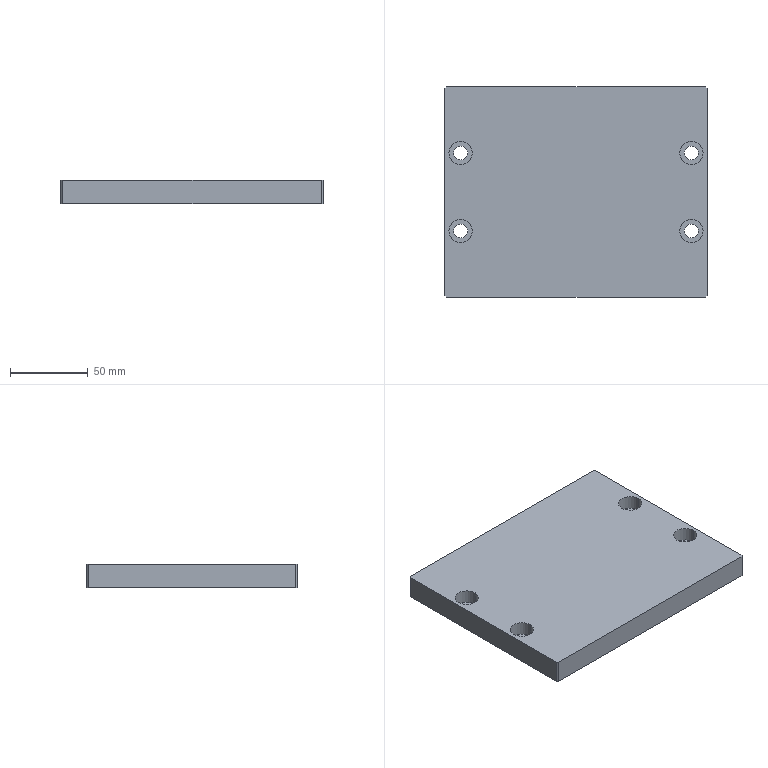Part | SolidWorks | features Chamfer 1, Extrusion 1, HoleWzd 1 | 1 solid | 30 faces | box 168 x 135 x 15 mm | volume 332281 mm3 | cylinder 16 | plane 14 | commonest cylinder face diameters 9 x8 15 x8
STEP:
#1=CARTESIAN_POINT('',(-81.5,25.,6.));
#2=VERTEX_POINT('',#1);
#3=CARTESIAN_POINT('',(-66.5,25.,6.));
#4=VERTEX_POINT('',#3);
#5=CARTESIAN_POINT('',(-74.,25.,6.));
#6=DIRECTION('',(0.,0.,1.));
#7=DIRECTION('',(1.,0.,0.));
#8=AXIS2_PLACEMENT_3D('',#5,#6,#7);
#9=CIRCLE('',#8,7.5);
#10=EDGE_CURVE('',#2,#4,#9,.T.);
#11=ORIENTED_EDGE('',*,*,#10,.F.);
#12=CARTESIAN_POINT('',(-81.5,25.,15.));
#13=VERTEX_POINT('',#12);
#14=CARTESIAN_POINT('',(-81.5,25.,15.));
#15=DIRECTION('',(0.,0.,1.));
#16=VECTOR('',#15,1000.);
#17=LINE('',#14,#16);
#18=EDGE_CURVE('',#2,#13,#17,.T.);
#19=ORIENTED_EDGE('',*,*,#18,.T.);
#20=CARTESIAN_POINT('',(-66.5,25.,15.));
#21=VERTEX_POINT('',#20);
#22=CARTESIAN_POINT('',(-74.,25.,15.));
#23=DIRECTION('',(0.,0.,1.));
#24=DIRECTION('',(1.,0.,0.));
#25=AXIS2_PLACEMENT_3D('',#22,#23,#24);
#26=CIRCLE('',#25,7.5);
#27=EDGE_CURVE('',#13,#21,#26,.T.);
#28=ORIENTED_EDGE('',*,*,#27,.T.);
#29=CARTESIAN_POINT('',(-66.5,25.,15.));
#30=DIRECTION('',(0.,0.,1.));
#31=VECTOR('',#30,1000.);
#32=LINE('',#29,#31);
#33=EDGE_CURVE('',#4,#21,#32,.T.);
#34=ORIENTED_EDGE('',*,*,#33,.F.);
#35=EDGE_LOOP('',(#11,#19,#28,#34));
#36=FACE_OUTER_BOUND('',#35,.T.);
#37=CARTESIAN_POINT('',(-74.,25.,15.));
#38=DIRECTION('',(0.,0.,1.));
#39=DIRECTION('',(1.,0.,0.));
#40=AXIS2_PLACEMENT_3D('',#37,#38,#39);
#41=CYLINDRICAL_SURFACE('',#40,7.5);
#42=ADVANCED_FACE('',(#36),#41,.F.);
#43=CARTESIAN_POINT('',(-78.5,25.,0.));
#44=VERTEX_POINT('',#43);
#45=CARTESIAN_POINT('',(-69.5,25.,0.));
#46=VERTEX_POINT('',#45);
#47=CARTESIAN_POINT('',(-74.,25.,0.));
#48=DIRECTION('',(0.,0.,1.));
#49=DIRECTION('',(1.,0.,0.));
#50=AXIS2_PLACEMENT_3D('',#47,#48,#49);
#51=CIRCLE('',#50,4.5);
#52=EDGE_CURVE('',#44,#46,#51,.T.);
#53=ORIENTED_EDGE('',*,*,#52,.F.);
#54=CARTESIAN_POINT('',(-78.5,25.,6.));
#55=VERTEX_POINT('',#54);
#56=CARTESIAN_POINT('',(-78.5,25.,15.));
#57=DIRECTION('',(0.,0.,1.));
#58=VECTOR('',#57,1000.);
#59=LINE('',#56,#58);
#60=EDGE_CURVE('',#44,#55,#59,.T.);
#61=ORIENTED_EDGE('',*,*,#60,.T.);
#62=CARTESIAN_POINT('',(-69.5,25.,6.));
#63=VERTEX_POINT('',#62);
#64=CARTESIAN_POINT('',(-74.,25.,6.));
#65=DIRECTION('',(0.,0.,1.));
#66=DIRECTION('',(1.,0.,0.));
#67=AXIS2_PLACEMENT_3D('',#64,#65,#66);
#68=CIRCLE('',#67,4.5);
#69=EDGE_CURVE('',#55,#63,#68,.T.);
#70=ORIENTED_EDGE('',*,*,#69,.T.);
#71=CARTESIAN_POINT('',(-69.5,25.,15.));
#72=DIRECTION('',(0.,0.,1.));
#73=VECTOR('',#72,1000.);
#74=LINE('',#71,#73);
#75=EDGE_CURVE('',#46,#63,#74,.T.);
#76=ORIENTED_EDGE('',*,*,#75,.F.);
#77=EDGE_LOOP('',(#53,#61,#70,#76));
#78=FACE_OUTER_BOUND('',#77,.T.);
#79=CARTESIAN_POINT('',(-74.,25.,15.));
#80=DIRECTION('',(0.,0.,1.));
#81=DIRECTION('',(1.,0.,0.));
#82=AXIS2_PLACEMENT_3D('',#79,#80,#81);
#83=CYLINDRICAL_SURFACE('',#82,4.5);
#84=ADVANCED_FACE('',(#78),#83,.F.);
#85=CARTESIAN_POINT('',(-81.5,-25.,6.));
#86=VERTEX_POINT('',#85);
#87=CARTESIAN_POINT('',(-66.5,-25.,6.));
#88=VERTEX_POINT('',#87);
#89=CARTESIAN_POINT('',(-74.,-25.,6.));
#90=DIRECTION('',(0.,0.,1.));
#91=DIRECTION('',(1.,0.,0.));
#92=AXIS2_PLACEMENT_3D('',#89,#90,#91);
#93=CIRCLE('',#92,7.5);
#94=EDGE_CURVE('',#86,#88,#93,.T.);
#95=ORIENTED_EDGE('',*,*,#94,.F.);
#96=CARTESIAN_POINT('',(-81.5,-25.,15.));
#97=VERTEX_POINT('',#96);
#98=CARTESIAN_POINT('',(-81.5,-25.,15.));
#99=DIRECTION('',(0.,0.,1.));
#100=VECTOR('',#99,1000.);
#101=LINE('',#98,#100);
#102=EDGE_CURVE('',#86,#97,#101,.T.);
#103=ORIENTED_EDGE('',*,*,#102,.T.);
#104=CARTESIAN_POINT('',(-66.5,-25.,15.));
#105=VERTEX_POINT('',#104);
#106=CARTESIAN_POINT('',(-74.,-25.,15.));
#107=DIRECTION('',(0.,0.,1.));
#108=DIRECTION('',(1.,0.,0.));
#109=AXIS2_PLACEMENT_3D('',#106,#107,#108);
#110=CIRCLE('',#109,7.5);
#111=EDGE_CURVE('',#97,#105,#110,.T.);
#112=ORIENTED_EDGE('',*,*,#111,.T.);
#113=CARTESIAN_POINT('',(-66.5,-25.,15.));
#114=DIRECTION('',(0.,0.,1.));
#115=VECTOR('',#114,1000.);
#116=LINE('',#113,#115);
#117=EDGE_CURVE('',#88,#105,#116,.T.);
#118=ORIENTED_EDGE('',*,*,#117,.F.);
#119=EDGE_LOOP('',(#95,#103,#112,#118));
#120=FACE_OUTER_BOUND('',#119,.T.);
#121=CARTESIAN_POINT('',(-74.,-25.,15.));
#122=DIRECTION('',(0.,0.,1.));
#123=DIRECTION('',(1.,0.,0.));
#124=AXIS2_PLACEMENT_3D('',#121,#122,#123);
#125=CYLINDRICAL_SURFACE('',#124,7.5);
#126=ADVANCED_FACE('',(#120),#125,.F.);
#127=CARTESIAN_POINT('',(-78.5,-25.,0.));
#128=VERTEX_POINT('',#127);
#129=CARTESIAN_POINT('',(-69.5,-25.,0.));
#130=VERTEX_POINT('',#129);
#131=CARTESIAN_POINT('',(-74.,-25.,0.));
#132=DIRECTION('',(0.,0.,1.));
#133=DIRECTION('',(1.,0.,0.));
#134=AXIS2_PLACEMENT_3D('',#131,#132,#133);
#135=CIRCLE('',#134,4.5);
#136=EDGE_CURVE('',#128,#130,#135,.T.);
#137=ORIENTED_EDGE('',*,*,#136,.F.);
#138=CARTESIAN_POINT('',(-78.5,-25.,6.));
#139=VERTEX_POINT('',#138);
#140=CARTESIAN_POINT('',(-78.5,-25.,15.));
#141=DIRECTION('',(0.,0.,1.));
#142=VECTOR('',#141,1000.);
#143=LINE('',#140,#142);
#144=EDGE_CURVE('',#128,#139,#143,.T.);
#145=ORIENTED_EDGE('',*,*,#144,.T.);
#146=CARTESIAN_POINT('',(-69.5,-25.,6.));
#147=VERTEX_POINT('',#146);
#148=CARTESIAN_POINT('',(-74.,-25.,6.));
#149=DIRECTION('',(0.,0.,1.));
#150=DIRECTION('',(1.,0.,0.));
#151=AXIS2_PLACEMENT_3D('',#148,#149,#150);
#152=CIRCLE('',#151,4.5);
#153=EDGE_CURVE('',#139,#147,#152,.T.);
#154=ORIENTED_EDGE('',*,*,#153,.T.);
#155=CARTESIAN_POINT('',(-69.5,-25.,15.));
#156=DIRECTION('',(0.,0.,1.));
#157=VECTOR('',#156,1000.);
#158=LINE('',#155,#157);
#159=EDGE_CURVE('',#130,#147,#158,.T.);
#160=ORIENTED_EDGE('',*,*,#159,.F.);
#161=EDGE_LOOP('',(#137,#145,#154,#160));
#162=FACE_OUTER_BOUND('',#161,.T.);
#163=CARTESIAN_POINT('',(-74.,-25.,15.));
#164=DIRECTION('',(0.,0.,1.));
#165=DIRECTION('',(1.,0.,0.));
#166=AXIS2_PLACEMENT_3D('',#163,#164,#165);
#167=CYLINDRICAL_SURFACE('',#166,4.5);
#168=ADVANCED_FACE('',(#162),#167,.F.);
#169=CARTESIAN_POINT('',(66.5,-25.,6.));
#170=VERTEX_POINT('',#169);
#171=CARTESIAN_POINT('',(81.5,-25.,6.));
#172=VERTEX_POINT('',#171);
#173=CARTESIAN_POINT('',(74.,-25.,6.));
#174=DIRECTION('',(0.,0.,1.));
#175=DIRECTION('',(1.,0.,0.));
#176=AXIS2_PLACEMENT_3D('',#173,#174,#175);
#177=CIRCLE('',#176,7.5);
#178=EDGE_CURVE('',#170,#172,#177,.T.);
#179=ORIENTED_EDGE('',*,*,#178,.F.);
#180=CARTESIAN_POINT('',(66.5,-25.,15.));
#181=VERTEX_POINT('',#180);
#182=CARTESIAN_POINT('',(66.5,-25.,15.));
#183=DIRECTION('',(0.,0.,1.));
#184=VECTOR('',#183,1000.);
#185=LINE('',#182,#184);
#186=EDGE_CURVE('',#170,#181,#185,.T.);
#187=ORIENTED_EDGE('',*,*,#186,.T.);
#188=CARTESIAN_POINT('',(81.5,-25.,15.));
#189=VERTEX_POINT('',#188);
#190=CARTESIAN_POINT('',(74.,-25.,15.));
#191=DIRECTION('',(0.,0.,1.));
#192=DIRECTION('',(1.,0.,0.));
#193=AXIS2_PLACEMENT_3D('',#190,#191,#192);
#194=CIRCLE('',#193,7.5);
#195=EDGE_CURVE('',#181,#189,#194,.T.);
#196=ORIENTED_EDGE('',*,*,#195,.T.);
#197=CARTESIAN_POINT('',(81.5,-25.,15.));
#198=DIRECTION('',(0.,0.,1.));
#199=VECTOR('',#198,1000.);
#200=LINE('',#197,#199);
#201=EDGE_CURVE('',#172,#189,#200,.T.);
#202=ORIENTED_EDGE('',*,*,#201,.F.);
#203=EDGE_LOOP('',(#179,#187,#196,#202));
#204=FACE_OUTER_BOUND('',#203,.T.);
#205=CARTESIAN_POINT('',(74.,-25.,15.));
#206=DIRECTION('',(0.,0.,1.));
#207=DIRECTION('',(1.,0.,0.));
#208=AXIS2_PLACEMENT_3D('',#205,#206,#207);
#209=CYLINDRICAL_SURFACE('',#208,7.5);
#210=ADVANCED_FACE('',(#204),#209,.F.);
#211=CARTESIAN_POINT('',(69.5,-25.,0.));
#212=VERTEX_POINT('',#211);
#213=CARTESIAN_POINT('',(78.5,-25.,0.));
#214=VERTEX_POINT('',#213);
#215=CARTESIAN_POINT('',(74.,-25.,0.));
#216=DIRECTION('',(0.,0.,1.));
#217=DIRECTION('',(1.,0.,0.));
#218=AXIS2_PLACEMENT_3D('',#215,#216,#217);
#219=CIRCLE('',#218,4.5);
#220=EDGE_CURVE('',#212,#214,#219,.T.);
#221=ORIENTED_EDGE('',*,*,#220,.F.);
#222=CARTESIAN_POINT('',(69.5,-25.,6.));
#223=VERTEX_POINT('',#222);
#224=CARTESIAN_POINT('',(69.5,-25.,15.));
#225=DIRECTION('',(0.,0.,1.));
#226=VECTOR('',#225,1000.);
#227=LINE('',#224,#226);
#228=EDGE_CURVE('',#212,#223,#227,.T.);
#229=ORIENTED_EDGE('',*,*,#228,.T.);
#230=CARTESIAN_POINT('',(78.5,-25.,6.));
#231=VERTEX_POINT('',#230);
#232=CARTESIAN_POINT('',(74.,-25.,6.));
#233=DIRECTION('',(0.,0.,1.));
#234=DIRECTION('',(1.,0.,0.));
#235=AXIS2_PLACEMENT_3D('',#232,#233,#234);
#236=CIRCLE('',#235,4.5);
#237=EDGE_CURVE('',#223,#231,#236,.T.);
#238=ORIENTED_EDGE('',*,*,#237,.T.);
#239=CARTESIAN_POINT('',(78.5,-25.,15.));
#240=DIRECTION('',(0.,0.,1.));
#241=VECTOR('',#240,1000.);
#242=LINE('',#239,#241);
#243=EDGE_CURVE('',#214,#231,#242,.T.);
#244=ORIENTED_EDGE('',*,*,#243,.F.);
#245=EDGE_LOOP('',(#221,#229,#238,#244));
#246=FACE_OUTER_BOUND('',#245,.T.);
#247=CARTESIAN_POINT('',(74.,-25.,15.));
#248=DIRECTION('',(0.,0.,1.));
#249=DIRECTION('',(1.,0.,0.));
#250=AXIS2_PLACEMENT_3D('',#247,#248,#249);
#251=CYLINDRICAL_SURFACE('',#250,4.5);
#252=ADVANCED_FACE('',(#246),#251,.F.);
#253=CARTESIAN_POINT('',(66.5,25.,6.));
#254=VERTEX_POINT('',#253);
#255=CARTESIAN_POINT('',(81.5,25.,6.));
#256=VERTEX_POINT('',#255);
#257=CARTESIAN_POINT('',(74.,25.,6.));
#258=DIRECTION('',(0.,0.,1.));
#259=DIRECTION('',(1.,0.,0.));
#260=AXIS2_PLACEMENT_3D('',#257,#258,#259);
#261=CIRCLE('',#260,7.5);
#262=EDGE_CURVE('',#254,#256,#261,.T.);
#263=ORIENTED_EDGE('',*,*,#262,.F.);
#264=CARTESIAN_POINT('',(66.5,25.,15.));
#265=VERTEX_POINT('',#264);
#266=CARTESIAN_POINT('',(66.5,25.,15.));
#267=DIRECTION('',(0.,0.,1.));
#268=VECTOR('',#267,1000.);
#269=LINE('',#266,#268);
#270=EDGE_CURVE('',#254,#265,#269,.T.);
#271=ORIENTED_EDGE('',*,*,#270,.T.);
#272=CARTESIAN_POINT('',(81.5,25.,15.));
#273=VERTEX_POINT('',#272);
#274=CARTESIAN_POINT('',(74.,25.,15.));
#275=DIRECTION('',(0.,0.,1.));
#276=DIRECTION('',(1.,0.,0.));
#277=AXIS2_PLACEMENT_3D('',#274,#275,#276);
#278=CIRCLE('',#277,7.5);
#279=EDGE_CURVE('',#265,#273,#278,.T.);
#280=ORIENTED_EDGE('',*,*,#279,.T.);
#281=CARTESIAN_POINT('',(81.5,25.,15.));
#282=DIRECTION('',(0.,0.,1.));
#283=VECTOR('',#282,1000.);
#284=LINE('',#281,#283);
#285=EDGE_CURVE('',#256,#273,#284,.T.);
#286=ORIENTED_EDGE('',*,*,#285,.F.);
#287=EDGE_LOOP('',(#263,#271,#280,#286));
#288=FACE_OUTER_BOUND('',#287,.T.);
#289=CARTESIAN_POINT('',(74.,25.,15.));
#290=DIRECTION('',(0.,0.,1.));
#291=DIRECTION('',(1.,0.,0.));
#292=AXIS2_PLACEMENT_3D('',#289,#290,#291);
#293=CYLINDRICAL_SURFACE('',#292,7.5);
#294=ADVANCED_FACE('',(#288),#293,.F.);
#295=CARTESIAN_POINT('',(69.5,25.,0.));
#296=VERTEX_POINT('',#295);
#297=CARTESIAN_POINT('',(78.5,25.,0.));
#298=VERTEX_POINT('',#297);
#299=CARTESIAN_POINT('',(74.,25.,0.));
#300=DIRECTION('',(0.,0.,1.));
#301=DIRECTION('',(1.,0.,0.));
#302=AXIS2_PLACEMENT_3D('',#299,#300,#301);
#303=CIRCLE('',#302,4.5);
#304=EDGE_CURVE('',#296,#298,#303,.T.);
#305=ORIENTED_EDGE('',*,*,#304,.F.);
#306=CARTESIAN_POINT('',(69.5,25.,6.));
#307=VERTEX_POINT('',#306);
#308=CARTESIAN_POINT('',(69.5,25.,15.));
#309=DIRECTION('',(0.,0.,1.));
#310=VECTOR('',#309,1000.);
#311=LINE('',#308,#310);
#312=EDGE_CURVE('',#296,#307,#311,.T.);
#313=ORIENTED_EDGE('',*,*,#312,.T.);
#314=CARTESIAN_POINT('',(78.5,25.,6.));
#315=VERTEX_POINT('',#314);
#316=CARTESIAN_POINT('',(74.,25.,6.));
#317=DIRECTION('',(0.,0.,1.));
#318=DIRECTION('',(1.,0.,0.));
#319=AXIS2_PLACEMENT_3D('',#316,#317,#318);
#320=CIRCLE('',#319,4.5);
#321=EDGE_CURVE('',#307,#315,#320,.T.);
#322=ORIENTED_EDGE('',*,*,#321,.T.);
#323=CARTESIAN_POINT('',(78.5,25.,15.));
#324=DIRECTION('',(0.,0.,1.));
#325=VECTOR('',#324,1000.);
#326=LINE('',#323,#325);
#327=EDGE_CURVE('',#298,#315,#326,.T.);
#328=ORIENTED_EDGE('',*,*,#327,.F.);
#329=EDGE_LOOP('',(#305,#313,#322,#328));
#330=FACE_OUTER_BOUND('',#329,.T.);
#331=CARTESIAN_POINT('',(74.,25.,15.));
#332=DIRECTION('',(0.,0.,1.));
#333=DIRECTION('',(1.,0.,0.));
#334=AXIS2_PLACEMENT_3D('',#331,#332,#333);
#335=CYLINDRICAL_SURFACE('',#334,4.5);
#336=ADVANCED_FACE('',(#330),#335,.F.);
#337=CARTESIAN_POINT('',(84.,-66.5,0.));
#338=VERTEX_POINT('',#337);
#339=CARTESIAN_POINT('',(84.,66.5,0.));
#340=VERTEX_POINT('',#339);
#341=CARTESIAN_POINT('',(84.,67.5,0.));
#342=DIRECTION('',(0.,1.,0.));
#343=VECTOR('',#342,1000.);
#344=LINE('',#341,#343);
#345=EDGE_CURVE('',#338,#340,#344,.T.);
#346=ORIENTED_EDGE('',*,*,#345,.T.);
#347=CARTESIAN_POINT('',(84.,66.5,15.));
#348=VERTEX_POINT('',#347);
#349=CARTESIAN_POINT('',(84.,66.5,15.));
#350=DIRECTION('',(0.,0.,1.));
#351=VECTOR('',#350,1000.);
#352=LINE('',#349,#351);
#353=EDGE_CURVE('',#340,#348,#352,.T.);
#354=ORIENTED_EDGE('',*,*,#353,.T.);
#355=CARTESIAN_POINT('',(84.,-66.5,15.));
#356=VERTEX_POINT('',#355);
#357=CARTESIAN_POINT('',(84.,67.5,15.));
#358=DIRECTION('',(0.,1.,0.));
#359=VECTOR('',#358,1000.);
#360=LINE('',#357,#359);
#361=EDGE_CURVE('',#356,#348,#360,.T.);
#362=ORIENTED_EDGE('',*,*,#361,.F.);
#363=CARTESIAN_POINT('',(84.,-66.5,15.));
#364=DIRECTION('',(0.,0.,-1.));
#365=VECTOR('',#364,1000.);
#366=LINE('',#363,#365);
#367=EDGE_CURVE('',#356,#338,#366,.T.);
#368=ORIENTED_EDGE('',*,*,#367,.T.);
#369=EDGE_LOOP('',(#346,#354,#362,#368));
#370=FACE_OUTER_BOUND('',#369,.T.);
#371=CARTESIAN_POINT('',(84.,67.5,15.));
#372=DIRECTION('',(-1.,0.,0.));
#373=DIRECTION('',(0.,-1.,0.));
#374=AXIS2_PLACEMENT_3D('',#371,#372,#373);
#375=PLANE('',#374);
#376=ADVANCED_FACE('',(#370),#375,.F.);
#377=CARTESIAN_POINT('',(83.,67.5,0.));
#378=VERTEX_POINT('',#377);
#379=CARTESIAN_POINT('',(-83.,67.5,0.));
#380=VERTEX_POINT('',#379);
#381=CARTESIAN_POINT('',(-84.,67.5,0.));
#382=DIRECTION('',(-1.,0.,0.));
#383=VECTOR('',#382,1000.);
#384=LINE('',#381,#383);
#385=EDGE_CURVE('',#378,#380,#384,.T.);
#386=ORIENTED_EDGE('',*,*,#385,.T.);
#387=CARTESIAN_POINT('',(-83.,67.5,15.));
#388=VERTEX_POINT('',#387);
#389=CARTESIAN_POINT('',(-83.,67.5,15.));
#390=DIRECTION('',(0.,0.,1.));
#391=VECTOR('',#390,1000.);
#392=LINE('',#389,#391);
#393=EDGE_CURVE('',#380,#388,#392,.T.);
#394=ORIENTED_EDGE('',*,*,#393,.T.);
#395=CARTESIAN_POINT('',(83.,67.5,15.));
#396=VERTEX_POINT('',#395);
#397=CARTESIAN_POINT('',(-84.,67.5,15.));
#398=DIRECTION('',(-1.,0.,0.));
#399=VECTOR('',#398,1000.);
#400=LINE('',#397,#399);
#401=EDGE_CURVE('',#396,#388,#400,.T.);
#402=ORIENTED_EDGE('',*,*,#401,.F.);
#403=CARTESIAN_POINT('',(83.,67.5,15.));
#404=DIRECTION('',(0.,0.,-1.));
#405=VECTOR('',#404,1000.);
#406=LINE('',#403,#405);
#407=EDGE_CURVE('',#396,#378,#406,.T.);
#408=ORIENTED_EDGE('',*,*,#407,.T.);
#409=EDGE_LOOP('',(#386,#394,#402,#408));
#410=FACE_OUTER_BOUND('',#409,.T.);
#411=CARTESIAN_POINT('',(-84.,67.5,15.));
#412=DIRECTION('',(0.,-1.,0.));
#413=DIRECTION('',(0.,0.,-1.));
#414=AXIS2_PLACEMENT_3D('',#411,#412,#413);
#415=PLANE('',#414);
#416=ADVANCED_FACE('',(#410),#415,.F.);
#417=CARTESIAN_POINT('',(-84.,66.5,15.));
#418=VERTEX_POINT('',#417);
#419=CARTESIAN_POINT('',(-84.,-66.5,15.));
#420=VERTEX_POINT('',#419);
#421=CARTESIAN_POINT('',(-84.,67.5,15.));
#422=DIRECTION('',(0.,-1.,0.));
#423=VECTOR('',#422,1000.);
#424=LINE('',#421,#423);
#425=EDGE_CURVE('',#418,#420,#424,.T.);
#426=ORIENTED_EDGE('',*,*,#425,.F.);
#427=CARTESIAN_POINT('',(-84.,66.5,0.));
#428=VERTEX_POINT('',#427);
#429=CARTESIAN_POINT('',(-84.,66.5,15.));
#430=DIRECTION('',(0.,0.,-1.));
#431=VECTOR('',#430,1000.);
#432=LINE('',#429,#431);
#433=EDGE_CURVE('',#418,#428,#432,.T.);
#434=ORIENTED_EDGE('',*,*,#433,.T.);
#435=CARTESIAN_POINT('',(-84.,-66.5,0.));
#436=VERTEX_POINT('',#435);
#437=CARTESIAN_POINT('',(-84.,67.5,0.));
#438=DIRECTION('',(0.,-1.,0.));
#439=VECTOR('',#438,1000.);
#440=LINE('',#437,#439);
#441=EDGE_CURVE('',#428,#436,#440,.T.);
#442=ORIENTED_EDGE('',*,*,#441,.T.);
#443=CARTESIAN_POINT('',(-84.,-66.5,15.));
#444=DIRECTION('',(0.,0.,1.));
#445=VECTOR('',#444,1000.);
#446=LINE('',#443,#445);
#447=EDGE_CURVE('',#436,#420,#446,.T.);
#448=ORIENTED_EDGE('',*,*,#447,.T.);
#449=EDGE_LOOP('',(#426,#434,#442,#448));
#450=FACE_OUTER_BOUND('',#449,.T.);
#451=CARTESIAN_POINT('',(-84.,67.5,15.));
#452=DIRECTION('',(1.,0.,0.));
#453=DIRECTION('',(0.,1.,0.));
#454=AXIS2_PLACEMENT_3D('',#451,#452,#453);
#455=PLANE('',#454);
#456=ADVANCED_FACE('',(#450),#455,.F.);
#457=CARTESIAN_POINT('',(-83.,-67.5,0.));
#458=VERTEX_POINT('',#457);
#459=CARTESIAN_POINT('',(83.,-67.5,0.));
#460=VERTEX_POINT('',#459);
#461=CARTESIAN_POINT('',(-84.,-67.5,0.));
#462=DIRECTION('',(1.,0.,0.));
#463=VECTOR('',#462,1000.);
#464=LINE('',#461,#463);
#465=EDGE_CURVE('',#458,#460,#464,.T.);
#466=ORIENTED_EDGE('',*,*,#465,.T.);
#467=CARTESIAN_POINT('',(83.,-67.5,15.));
#468=VERTEX_POINT('',#467);
#469=CARTESIAN_POINT('',(83.,-67.5,15.));
#470=DIRECTION('',(0.,0.,1.));
#471=VECTOR('',#470,1000.);
#472=LINE('',#469,#471);
#473=EDGE_CURVE('',#460,#468,#472,.T.);
#474=ORIENTED_EDGE('',*,*,#473,.T.);
#475=CARTESIAN_POINT('',(-83.,-67.5,15.));
#476=VERTEX_POINT('',#475);
#477=CARTESIAN_POINT('',(-84.,-67.5,15.));
#478=DIRECTION('',(1.,0.,0.));
#479=VECTOR('',#478,1000.);
#480=LINE('',#477,#479);
#481=EDGE_CURVE('',#476,#468,#480,.T.);
#482=ORIENTED_EDGE('',*,*,#481,.F.);
#483=CARTESIAN_POINT('',(-83.,-67.5,15.));
#484=DIRECTION('',(0.,0.,-1.));
#485=VECTOR('',#484,1000.);
#486=LINE('',#483,#485);
#487=EDGE_CURVE('',#476,#458,#486,.T.);
#488=ORIENTED_EDGE('',*,*,#487,.T.);
#489=EDGE_LOOP('',(#466,#474,#482,#488));
#490=FACE_OUTER_BOUND('',#489,.T.);
#491=CARTESIAN_POINT('',(-84.,-67.5,15.));
#492=DIRECTION('',(0.,1.,0.));
#493=DIRECTION('',(0.,0.,1.));
#494=AXIS2_PLACEMENT_3D('',#491,#492,#493);
#495=PLANE('',#494);
#496=ADVANCED_FACE('',(#490),#495,.F.);
#497=CARTESIAN_POINT('',(-74.,25.,15.));
#498=DIRECTION('',(0.,0.,1.));
#499=DIRECTION('',(1.,0.,0.));
#500=AXIS2_PLACEMENT_3D('',#497,#498,#499);
#501=CIRCLE('',#500,7.5);
#502=EDGE_CURVE('',#21,#13,#501,.T.);
#503=ORIENTED_EDGE('',*,*,#502,.F.);
#504=ORIENTED_EDGE('',*,*,#27,.F.);
#505=EDGE_LOOP('',(#503,#504));
#506=FACE_BOUND('',#505,.T.);
#507=CARTESIAN_POINT('',(-74.,-25.,15.));
#508=DIRECTION('',(0.,0.,1.));
#509=DIRECTION('',(1.,0.,0.));
#510=AXIS2_PLACEMENT_3D('',#507,#508,#509);
#511=CIRCLE('',#510,7.5);
#512=EDGE_CURVE('',#105,#97,#511,.T.);
#513=ORIENTED_EDGE('',*,*,#512,.F.);
#514=ORIENTED_EDGE('',*,*,#111,.F.);
#515=EDGE_LOOP('',(#513,#514));
#516=FACE_BOUND('',#515,.T.);
#517=CARTESIAN_POINT('',(74.,-25.,15.));
#518=DIRECTION('',(0.,0.,1.));
#519=DIRECTION('',(1.,0.,0.));
#520=AXIS2_PLACEMENT_3D('',#517,#518,#519);
#521=CIRCLE('',#520,7.5);
#522=EDGE_CURVE('',#189,#181,#521,.T.);
#523=ORIENTED_EDGE('',*,*,#522,.F.);
#524=ORIENTED_EDGE('',*,*,#195,.F.);
#525=EDGE_LOOP('',(#523,#524));
#526=FACE_BOUND('',#525,.T.);
#527=CARTESIAN_POINT('',(74.,25.,15.));
#528=DIRECTION('',(0.,0.,1.));
#529=DIRECTION('',(1.,0.,0.));
#530=AXIS2_PLACEMENT_3D('',#527,#528,#529);
#531=CIRCLE('',#530,7.5);
#532=EDGE_CURVE('',#273,#265,#531,.T.);
#533=ORIENTED_EDGE('',*,*,#532,.F.);
#534=ORIENTED_EDGE('',*,*,#279,.F.);
#535=EDGE_LOOP('',(#533,#534));
#536=FACE_BOUND('',#535,.T.);
#537=ORIENTED_EDGE('',*,*,#401,.T.);
#538=CARTESIAN_POINT('',(-67.,83.5,15.));
#539=DIRECTION('',(-0.7071,-0.7071,0.));
#540=VECTOR('',#539,1000.);
#541=LINE('',#538,#540);
#542=EDGE_CURVE('',#388,#418,#541,.T.);
#543=ORIENTED_EDGE('',*,*,#542,.T.);
#544=ORIENTED_EDGE('',*,*,#425,.T.);
#545=CARTESIAN_POINT('',(0.5,-151.,15.));
#546=DIRECTION('',(0.7071,-0.7071,0.));
#547=VECTOR('',#546,1000.);
#548=LINE('',#545,#547);
#549=EDGE_CURVE('',#420,#476,#548,.T.);
#550=ORIENTED_EDGE('',*,*,#549,.T.);
#551=ORIENTED_EDGE('',*,*,#481,.T.);
#552=CARTESIAN_POINT('',(83.5,-67.,15.));
#553=DIRECTION('',(0.7071,0.7071,0.));
#554=VECTOR('',#553,1000.);
#555=LINE('',#552,#554);
#556=EDGE_CURVE('',#468,#356,#555,.T.);
#557=ORIENTED_EDGE('',*,*,#556,.T.);
#558=ORIENTED_EDGE('',*,*,#361,.T.);
#559=CARTESIAN_POINT('',(151.,-0.5,15.));
#560=DIRECTION('',(-0.7071,0.7071,0.));
#561=VECTOR('',#560,1000.);
#562=LINE('',#559,#561);
#563=EDGE_CURVE('',#348,#396,#562,.T.);
#564=ORIENTED_EDGE('',*,*,#563,.T.);
#565=EDGE_LOOP('',(#537,#543,#544,#550,#551,#557,#558,#564));
#566=FACE_OUTER_BOUND('',#565,.T.);
#567=CARTESIAN_POINT('',(84.,-67.5,15.));
#568=DIRECTION('',(0.,0.,1.));
#569=DIRECTION('',(1.,0.,0.));
#570=AXIS2_PLACEMENT_3D('',#567,#568,#569);
#571=PLANE('',#570);
#572=ADVANCED_FACE('',(#506,#516,#526,#536,#566),#571,.T.);
#573=CARTESIAN_POINT('',(-74.,25.,0.));
#574=DIRECTION('',(0.,0.,1.));
#575=DIRECTION('',(1.,0.,0.));
#576=AXIS2_PLACEMENT_3D('',#573,#574,#575);
#577=CIRCLE('',#576,4.5);
#578=EDGE_CURVE('',#46,#44,#577,.T.);
#579=ORIENTED_EDGE('',*,*,#578,.T.);
#580=ORIENTED_EDGE('',*,*,#52,.T.);
#581=EDGE_LOOP('',(#579,#580));
#582=FACE_BOUND('',#581,.T.);
#583=CARTESIAN_POINT('',(-74.,-25.,0.));
#584=DIRECTION('',(0.,0.,1.));
#585=DIRECTION('',(1.,0.,0.));
#586=AXIS2_PLACEMENT_3D('',#583,#584,#585);
#587=CIRCLE('',#586,4.5);
#588=EDGE_CURVE('',#130,#128,#587,.T.);
#589=ORIENTED_EDGE('',*,*,#588,.T.);
#590=ORIENTED_EDGE('',*,*,#136,.T.);
#591=EDGE_LOOP('',(#589,#590));
#592=FACE_BOUND('',#591,.T.);
#593=CARTESIAN_POINT('',(74.,-25.,0.));
#594=DIRECTION('',(0.,0.,1.));
#595=DIRECTION('',(1.,0.,0.));
#596=AXIS2_PLACEMENT_3D('',#593,#594,#595);
#597=CIRCLE('',#596,4.5);
#598=EDGE_CURVE('',#214,#212,#597,.T.);
#599=ORIENTED_EDGE('',*,*,#598,.T.);
#600=ORIENTED_EDGE('',*,*,#220,.T.);
#601=EDGE_LOOP('',(#599,#600));
#602=FACE_BOUND('',#601,.T.);
#603=CARTESIAN_POINT('',(74.,25.,0.));
#604=DIRECTION('',(0.,0.,1.));
#605=DIRECTION('',(1.,0.,0.));
#606=AXIS2_PLACEMENT_3D('',#603,#604,#605);
#607=CIRCLE('',#606,4.5);
#608=EDGE_CURVE('',#298,#296,#607,.T.);
#609=ORIENTED_EDGE('',*,*,#608,.T.);
#610=ORIENTED_EDGE('',*,*,#304,.T.);
#611=EDGE_LOOP('',(#609,#610));
#612=FACE_BOUND('',#611,.T.);
#613=ORIENTED_EDGE('',*,*,#441,.F.);
#614=CARTESIAN_POINT('',(-84.,66.5,0.));
#615=DIRECTION('',(0.7071,0.7071,0.));
#616=VECTOR('',#615,1000.);
#617=LINE('',#614,#616);
#618=EDGE_CURVE('',#428,#380,#617,.T.);
#619=ORIENTED_EDGE('',*,*,#618,.T.);
#620=ORIENTED_EDGE('',*,*,#385,.F.);
#621=CARTESIAN_POINT('',(83.,67.5,0.));
#622=DIRECTION('',(0.7071,-0.7071,0.));
#623=VECTOR('',#622,1000.);
#624=LINE('',#621,#623);
#625=EDGE_CURVE('',#378,#340,#624,.T.);
#626=ORIENTED_EDGE('',*,*,#625,.T.);
#627=ORIENTED_EDGE('',*,*,#345,.F.);
#628=CARTESIAN_POINT('',(84.,-66.5,0.));
#629=DIRECTION('',(-0.7071,-0.7071,0.));
#630=VECTOR('',#629,1000.);
#631=LINE('',#628,#630);
#632=EDGE_CURVE('',#338,#460,#631,.T.);
#633=ORIENTED_EDGE('',*,*,#632,.T.);
#634=ORIENTED_EDGE('',*,*,#465,.F.);
#635=CARTESIAN_POINT('',(-83.,-67.5,0.));
#636=DIRECTION('',(-0.7071,0.7071,0.));
#637=VECTOR('',#636,1000.);
#638=LINE('',#635,#637);
#639=EDGE_CURVE('',#458,#436,#638,.T.);
#640=ORIENTED_EDGE('',*,*,#639,.T.);
#641=EDGE_LOOP('',(#613,#619,#620,#626,#627,#633,#634,#640));
#642=FACE_OUTER_BOUND('',#641,.T.);
#643=CARTESIAN_POINT('',(84.,-67.5,0.));
#644=DIRECTION('',(0.,0.,1.));
#645=DIRECTION('',(1.,0.,0.));
#646=AXIS2_PLACEMENT_3D('',#643,#644,#645);
#647=PLANE('',#646);
#648=ADVANCED_FACE('',(#582,#592,#602,#612,#642),#647,.F.);
#649=ORIENTED_EDGE('',*,*,#312,.F.);
#650=ORIENTED_EDGE('',*,*,#608,.F.);
#651=ORIENTED_EDGE('',*,*,#327,.T.);
#652=CARTESIAN_POINT('',(74.,25.,6.));
#653=DIRECTION('',(0.,0.,1.));
#654=DIRECTION('',(1.,0.,0.));
#655=AXIS2_PLACEMENT_3D('',#652,#653,#654);
#656=CIRCLE('',#655,4.5);
#657=EDGE_CURVE('',#315,#307,#656,.T.);
#658=ORIENTED_EDGE('',*,*,#657,.T.);
#659=EDGE_LOOP('',(#649,#650,#651,#658));
#660=FACE_OUTER_BOUND('',#659,.T.);
#661=CARTESIAN_POINT('',(74.,25.,15.));
#662=DIRECTION('',(0.,0.,1.));
#663=DIRECTION('',(1.,0.,0.));
#664=AXIS2_PLACEMENT_3D('',#661,#662,#663);
#665=CYLINDRICAL_SURFACE('',#664,4.5);
#666=ADVANCED_FACE('',(#660),#665,.F.);
#667=ORIENTED_EDGE('',*,*,#657,.F.);
#668=ORIENTED_EDGE('',*,*,#321,.F.);
#669=EDGE_LOOP('',(#667,#668));
#670=FACE_BOUND('',#669,.T.);
#671=CARTESIAN_POINT('',(74.,25.,6.));
#672=DIRECTION('',(0.,0.,1.));
#673=DIRECTION('',(1.,0.,0.));
#674=AXIS2_PLACEMENT_3D('',#671,#672,#673);
#675=CIRCLE('',#674,7.5);
#676=EDGE_CURVE('',#256,#254,#675,.T.);
#677=ORIENTED_EDGE('',*,*,#676,.T.);
#678=ORIENTED_EDGE('',*,*,#262,.T.);
#679=EDGE_LOOP('',(#677,#678));
#680=FACE_OUTER_BOUND('',#679,.T.);
#681=CARTESIAN_POINT('',(78.5,25.,6.));
#682=DIRECTION('',(0.,0.,-1.));
#683=DIRECTION('',(-1.,0.,0.));
#684=AXIS2_PLACEMENT_3D('',#681,#682,#683);
#685=PLANE('',#684);
#686=ADVANCED_FACE('',(#670,#680),#685,.F.);
#687=ORIENTED_EDGE('',*,*,#270,.F.);
#688=ORIENTED_EDGE('',*,*,#676,.F.);
#689=ORIENTED_EDGE('',*,*,#285,.T.);
#690=ORIENTED_EDGE('',*,*,#532,.T.);
#691=EDGE_LOOP('',(#687,#688,#689,#690));
#692=FACE_OUTER_BOUND('',#691,.T.);
#693=CARTESIAN_POINT('',(74.,25.,15.));
#694=DIRECTION('',(0.,0.,1.));
#695=DIRECTION('',(1.,0.,0.));
#696=AXIS2_PLACEMENT_3D('',#693,#694,#695);
#697=CYLINDRICAL_SURFACE('',#696,7.5);
#698=ADVANCED_FACE('',(#692),#697,.F.);
#699=ORIENTED_EDGE('',*,*,#228,.F.);
#700=ORIENTED_EDGE('',*,*,#598,.F.);
#701=ORIENTED_EDGE('',*,*,#243,.T.);
#702=CARTESIAN_POINT('',(74.,-25.,6.));
#703=DIRECTION('',(0.,0.,1.));
#704=DIRECTION('',(1.,0.,0.));
#705=AXIS2_PLACEMENT_3D('',#702,#703,#704);
#706=CIRCLE('',#705,4.5);
#707=EDGE_CURVE('',#231,#223,#706,.T.);
#708=ORIENTED_EDGE('',*,*,#707,.T.);
#709=EDGE_LOOP('',(#699,#700,#701,#708));
#710=FACE_OUTER_BOUND('',#709,.T.);
#711=CARTESIAN_POINT('',(74.,-25.,15.));
#712=DIRECTION('',(0.,0.,1.));
#713=DIRECTION('',(1.,0.,0.));
#714=AXIS2_PLACEMENT_3D('',#711,#712,#713);
#715=CYLINDRICAL_SURFACE('',#714,4.5);
#716=ADVANCED_FACE('',(#710),#715,.F.);
#717=ORIENTED_EDGE('',*,*,#707,.F.);
#718=ORIENTED_EDGE('',*,*,#237,.F.);
#719=EDGE_LOOP('',(#717,#718));
#720=FACE_BOUND('',#719,.T.);
#721=CARTESIAN_POINT('',(74.,-25.,6.));
#722=DIRECTION('',(0.,0.,1.));
#723=DIRECTION('',(1.,0.,0.));
#724=AXIS2_PLACEMENT_3D('',#721,#722,#723);
#725=CIRCLE('',#724,7.5);
#726=EDGE_CURVE('',#172,#170,#725,.T.);
#727=ORIENTED_EDGE('',*,*,#726,.T.);
#728=ORIENTED_EDGE('',*,*,#178,.T.);
#729=EDGE_LOOP('',(#727,#728));
#730=FACE_OUTER_BOUND('',#729,.T.);
#731=CARTESIAN_POINT('',(78.5,-25.,6.));
#732=DIRECTION('',(0.,0.,-1.));
#733=DIRECTION('',(-1.,0.,0.));
#734=AXIS2_PLACEMENT_3D('',#731,#732,#733);
#735=PLANE('',#734);
#736=ADVANCED_FACE('',(#720,#730),#735,.F.);
#737=ORIENTED_EDGE('',*,*,#186,.F.);
#738=ORIENTED_EDGE('',*,*,#726,.F.);
#739=ORIENTED_EDGE('',*,*,#201,.T.);
#740=ORIENTED_EDGE('',*,*,#522,.T.);
#741=EDGE_LOOP('',(#737,#738,#739,#740));
#742=FACE_OUTER_BOUND('',#741,.T.);
#743=CARTESIAN_POINT('',(74.,-25.,15.));
#744=DIRECTION('',(0.,0.,1.));
#745=DIRECTION('',(1.,0.,0.));
#746=AXIS2_PLACEMENT_3D('',#743,#744,#745);
#747=CYLINDRICAL_SURFACE('',#746,7.5);
#748=ADVANCED_FACE('',(#742),#747,.F.);
#749=ORIENTED_EDGE('',*,*,#144,.F.);
#750=ORIENTED_EDGE('',*,*,#588,.F.);
#751=ORIENTED_EDGE('',*,*,#159,.T.);
#752=CARTESIAN_POINT('',(-74.,-25.,6.));
#753=DIRECTION('',(0.,0.,1.));
#754=DIRECTION('',(1.,0.,0.));
#755=AXIS2_PLACEMENT_3D('',#752,#753,#754);
#756=CIRCLE('',#755,4.5);
#757=EDGE_CURVE('',#147,#139,#756,.T.);
#758=ORIENTED_EDGE('',*,*,#757,.T.);
#759=EDGE_LOOP('',(#749,#750,#751,#758));
#760=FACE_OUTER_BOUND('',#759,.T.);
#761=CARTESIAN_POINT('',(-74.,-25.,15.));
#762=DIRECTION('',(0.,0.,1.));
#763=DIRECTION('',(1.,0.,0.));
#764=AXIS2_PLACEMENT_3D('',#761,#762,#763);
#765=CYLINDRICAL_SURFACE('',#764,4.5);
#766=ADVANCED_FACE('',(#760),#765,.F.);
#767=ORIENTED_EDGE('',*,*,#757,.F.);
#768=ORIENTED_EDGE('',*,*,#153,.F.);
#769=EDGE_LOOP('',(#767,#768));
#770=FACE_BOUND('',#769,.T.);
#771=CARTESIAN_POINT('',(-74.,-25.,6.));
#772=DIRECTION('',(0.,0.,1.));
#773=DIRECTION('',(1.,0.,0.));
#774=AXIS2_PLACEMENT_3D('',#771,#772,#773);
#775=CIRCLE('',#774,7.5);
#776=EDGE_CURVE('',#88,#86,#775,.T.);
#777=ORIENTED_EDGE('',*,*,#776,.T.);
#778=ORIENTED_EDGE('',*,*,#94,.T.);
#779=EDGE_LOOP('',(#777,#778));
#780=FACE_OUTER_BOUND('',#779,.T.);
#781=CARTESIAN_POINT('',(-69.5,-25.,6.));
#782=DIRECTION('',(0.,0.,-1.));
#783=DIRECTION('',(-1.,0.,0.));
#784=AXIS2_PLACEMENT_3D('',#781,#782,#783);
#785=PLANE('',#784);
#786=ADVANCED_FACE('',(#770,#780),#785,.F.);
#787=ORIENTED_EDGE('',*,*,#102,.F.);
#788=ORIENTED_EDGE('',*,*,#776,.F.);
#789=ORIENTED_EDGE('',*,*,#117,.T.);
#790=ORIENTED_EDGE('',*,*,#512,.T.);
#791=EDGE_LOOP('',(#787,#788,#789,#790));
#792=FACE_OUTER_BOUND('',#791,.T.);
#793=CARTESIAN_POINT('',(-74.,-25.,15.));
#794=DIRECTION('',(0.,0.,1.));
#795=DIRECTION('',(1.,0.,0.));
#796=AXIS2_PLACEMENT_3D('',#793,#794,#795);
#797=CYLINDRICAL_SURFACE('',#796,7.5);
#798=ADVANCED_FACE('',(#792),#797,.F.);
#799=ORIENTED_EDGE('',*,*,#60,.F.);
#800=ORIENTED_EDGE('',*,*,#578,.F.);
#801=ORIENTED_EDGE('',*,*,#75,.T.);
#802=CARTESIAN_POINT('',(-74.,25.,6.));
#803=DIRECTION('',(0.,0.,1.));
#804=DIRECTION('',(1.,0.,0.));
#805=AXIS2_PLACEMENT_3D('',#802,#803,#804);
#806=CIRCLE('',#805,4.5);
#807=EDGE_CURVE('',#63,#55,#806,.T.);
#808=ORIENTED_EDGE('',*,*,#807,.T.);
#809=EDGE_LOOP('',(#799,#800,#801,#808));
#810=FACE_OUTER_BOUND('',#809,.T.);
#811=CARTESIAN_POINT('',(-74.,25.,15.));
#812=DIRECTION('',(0.,0.,1.));
#813=DIRECTION('',(1.,0.,0.));
#814=AXIS2_PLACEMENT_3D('',#811,#812,#813);
#815=CYLINDRICAL_SURFACE('',#814,4.5);
#816=ADVANCED_FACE('',(#810),#815,.F.);
#817=ORIENTED_EDGE('',*,*,#807,.F.);
#818=ORIENTED_EDGE('',*,*,#69,.F.);
#819=EDGE_LOOP('',(#817,#818));
#820=FACE_BOUND('',#819,.T.);
#821=CARTESIAN_POINT('',(-74.,25.,6.));
#822=DIRECTION('',(0.,0.,1.));
#823=DIRECTION('',(1.,0.,0.));
#824=AXIS2_PLACEMENT_3D('',#821,#822,#823);
#825=CIRCLE('',#824,7.5);
#826=EDGE_CURVE('',#4,#2,#825,.T.);
#827=ORIENTED_EDGE('',*,*,#826,.T.);
#828=ORIENTED_EDGE('',*,*,#10,.T.);
#829=EDGE_LOOP('',(#827,#828));
#830=FACE_OUTER_BOUND('',#829,.T.);
#831=CARTESIAN_POINT('',(-69.5,25.,6.));
#832=DIRECTION('',(0.,0.,-1.));
#833=DIRECTION('',(-1.,0.,0.));
#834=AXIS2_PLACEMENT_3D('',#831,#832,#833);
#835=PLANE('',#834);
#836=ADVANCED_FACE('',(#820,#830),#835,.F.);
#837=ORIENTED_EDGE('',*,*,#18,.F.);
#838=ORIENTED_EDGE('',*,*,#826,.F.);
#839=ORIENTED_EDGE('',*,*,#33,.T.);
#840=ORIENTED_EDGE('',*,*,#502,.T.);
#841=EDGE_LOOP('',(#837,#838,#839,#840));
#842=FACE_OUTER_BOUND('',#841,.T.);
#843=CARTESIAN_POINT('',(-74.,25.,15.));
#844=DIRECTION('',(0.,0.,1.));
#845=DIRECTION('',(1.,0.,0.));
#846=AXIS2_PLACEMENT_3D('',#843,#844,#845);
#847=CYLINDRICAL_SURFACE('',#846,7.5);
#848=ADVANCED_FACE('',(#842),#847,.F.);
#849=ORIENTED_EDGE('',*,*,#542,.F.);
#850=ORIENTED_EDGE('',*,*,#393,.F.);
#851=ORIENTED_EDGE('',*,*,#618,.F.);
#852=ORIENTED_EDGE('',*,*,#433,.F.);
#853=EDGE_LOOP('',(#849,#850,#851,#852));
#854=FACE_OUTER_BOUND('',#853,.T.);
#855=CARTESIAN_POINT('',(-84.,66.5,15.));
#856=DIRECTION('',(0.7071,-0.7071,0.));
#857=DIRECTION('',(0.7071,0.7071,0.));
#858=AXIS2_PLACEMENT_3D('',#855,#856,#857);
#859=PLANE('',#858);
#860=ADVANCED_FACE('',(#854),#859,.F.);
#861=ORIENTED_EDGE('',*,*,#563,.F.);
#862=ORIENTED_EDGE('',*,*,#353,.F.);
#863=ORIENTED_EDGE('',*,*,#625,.F.);
#864=ORIENTED_EDGE('',*,*,#407,.F.);
#865=EDGE_LOOP('',(#861,#862,#863,#864));
#866=FACE_OUTER_BOUND('',#865,.T.);
#867=CARTESIAN_POINT('',(83.,67.5,15.));
#868=DIRECTION('',(-0.7071,-0.7071,0.));
#869=DIRECTION('',(0.7071,-0.7071,0.));
#870=AXIS2_PLACEMENT_3D('',#867,#868,#869);
#871=PLANE('',#870);
#872=ADVANCED_FACE('',(#866),#871,.F.);
#873=ORIENTED_EDGE('',*,*,#556,.F.);
#874=ORIENTED_EDGE('',*,*,#473,.F.);
#875=ORIENTED_EDGE('',*,*,#632,.F.);
#876=ORIENTED_EDGE('',*,*,#367,.F.);
#877=EDGE_LOOP('',(#873,#874,#875,#876));
#878=FACE_OUTER_BOUND('',#877,.T.);
#879=CARTESIAN_POINT('',(84.,-66.5,15.));
#880=DIRECTION('',(-0.7071,0.7071,0.));
#881=DIRECTION('',(-0.7071,-0.7071,0.));
#882=AXIS2_PLACEMENT_3D('',#879,#880,#881);
#883=PLANE('',#882);
#884=ADVANCED_FACE('',(#878),#883,.F.);
#885=ORIENTED_EDGE('',*,*,#549,.F.);
#886=ORIENTED_EDGE('',*,*,#447,.F.);
#887=ORIENTED_EDGE('',*,*,#639,.F.);
#888=ORIENTED_EDGE('',*,*,#487,.F.);
#889=EDGE_LOOP('',(#885,#886,#887,#888));
#890=FACE_OUTER_BOUND('',#889,.T.);
#891=CARTESIAN_POINT('',(-83.,-67.5,15.));
#892=DIRECTION('',(0.7071,0.7071,0.));
#893=DIRECTION('',(-0.7071,0.7071,0.));
#894=AXIS2_PLACEMENT_3D('',#891,#892,#893);
#895=PLANE('',#894);
#896=ADVANCED_FACE('',(#890),#895,.F.);
#897=CLOSED_SHELL('',(#42,#84,#126,#168,#210,#252,#294,#336,#376,#416,#456,#496,#572,#648,#666,#686,#698,#716,#736,#748,#766,#786,#798,#816,#836,#848,#860,#872,#884,#896));
#898=MANIFOLD_SOLID_BREP('',#897);
#899=CARTESIAN_POINT('',(0.,0.,0.));
#900=DIRECTION('',(0.,0.,1.));
#901=DIRECTION('',(1.,0.,0.));
#902=AXIS2_PLACEMENT_3D('',#899,#900,#901);
#903=(LENGTH_UNIT()NAMED_UNIT(*)SI_UNIT(.MILLI.,.METRE.));
#904=UNCERTAINTY_MEASURE_WITH_UNIT(LENGTH_MEASURE(0.00001),#903,'','');
#905=(NAMED_UNIT(*)PLANE_ANGLE_UNIT()SI_UNIT($,.RADIAN.));
#906=(NAMED_UNIT(*)SI_UNIT($,.STERADIAN.)SOLID_ANGLE_UNIT());
#907=(GEOMETRIC_REPRESENTATION_CONTEXT(3)GLOBAL_UNCERTAINTY_ASSIGNED_CONTEXT((#904))GLOBAL_UNIT_ASSIGNED_CONTEXT((#903,#905,#906))REPRESENTATION_CONTEXT('',''));
#908=ADVANCED_BREP_SHAPE_REPRESENTATION('',(#898,#902),#907);